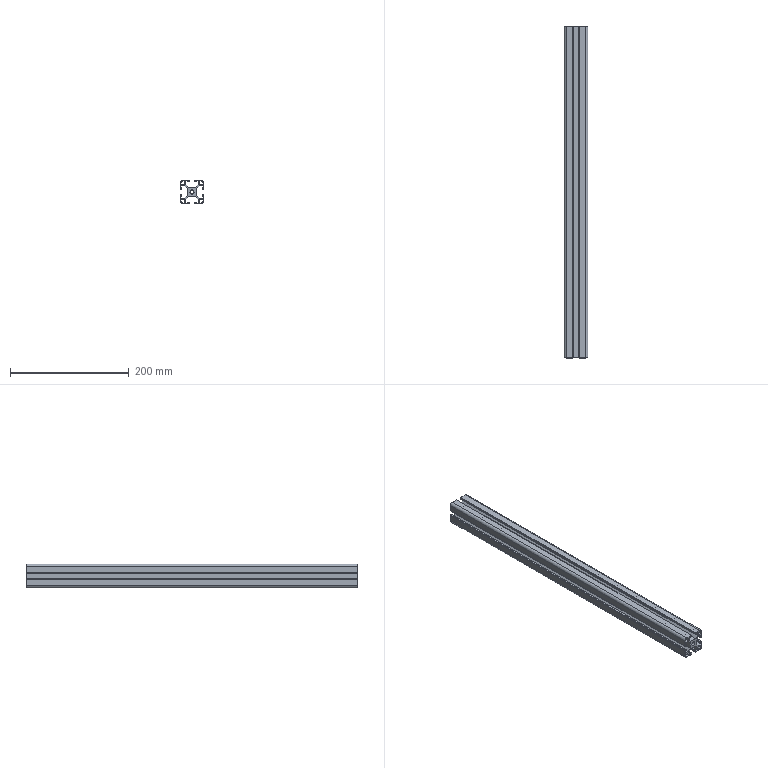Part | SolidWorks | features BaseBody 1 | 1 solid | 104 faces | box 40 x 560 x 40 mm | volume 322865 mm3 | plane 94 | cylinder 10 | commonest cylinder face diameters 5 x4 9 x4 6.8 x2